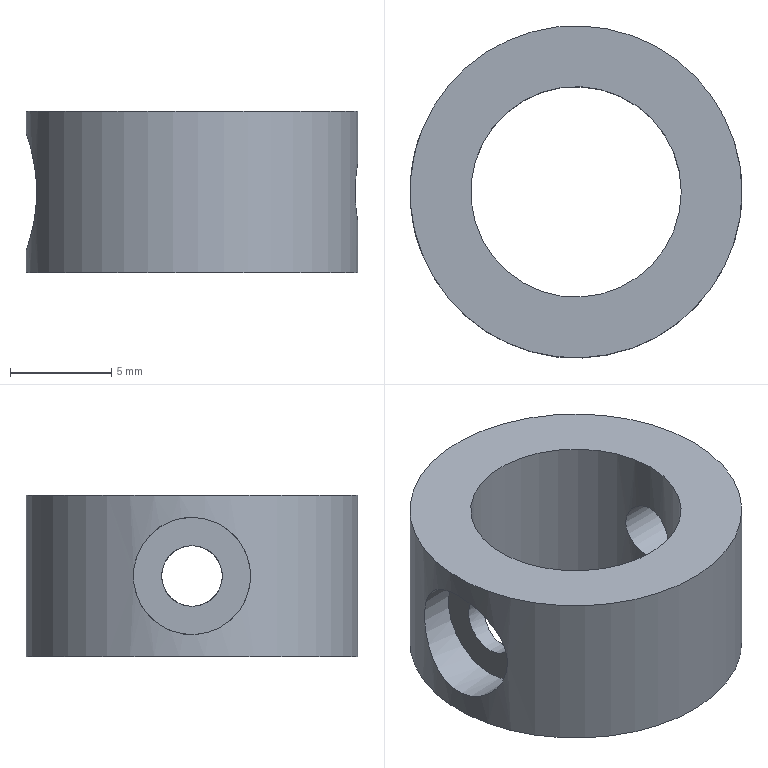Part | NX | features BREP 1, DATUM_CSYS 1 | 1 solid | 8 faces | box 16.4 x 16.4 x 8 mm | volume 928.38 mm3 | cylinder 5 | plane 3 | commonest cylinder face diameters 3 x2 5.8 x1 10.4 x1 16.4 x1
STEP:
#1=CARTESIAN_POINT('',(-6.,0.00000167,23.5));
#2=VERTEX_POINT('',#1);
#3=CARTESIAN_POINT('',(-6.,0.00000167,25.));
#4=DIRECTION('',(1.,0.,0.));
#5=DIRECTION('',(0.,0.,-1.));
#6=AXIS2_PLACEMENT_3D('',#3,#4,#5);
#7=CIRCLE('',#6,1.5);
#8=EDGE_CURVE('',#2,#2,#7,.T.);
#9=ORIENTED_EDGE('',*,*,#8,.F.);
#10=EDGE_LOOP('',(#9));
#11=FACE_BOUND('',#10,.T.);
#12=CARTESIAN_POINT('',(-5.2,-0.00002035,26.5));
#13=VERTEX_POINT('',#12);
#14=CARTESIAN_POINT('',(-5.092,-1.176,26.175));
#15=CARTESIAN_POINT('',(-5.254,0.0001171,26.663));
#16=CARTESIAN_POINT('',(-5.092,1.176,26.175));
#17=CARTESIAN_POINT('',(-4.922,1.662,25.002));
#18=CARTESIAN_POINT('',(-5.092,1.175,23.824));
#19=CARTESIAN_POINT('',(-5.254,0.0008864,23.338));
#20=CARTESIAN_POINT('',(-5.092,-1.175,23.824));
#21=CARTESIAN_POINT('',(-4.922,-1.662,25.));
#22=CARTESIAN_POINT('',(-5.092,-1.176,26.175));
#23=CARTESIAN_POINT('',(-5.254,0.0001171,26.663));
#24=CARTESIAN_POINT('',(-5.092,1.176,26.175));
#25=B_SPLINE_CURVE_WITH_KNOTS('',3,(#14,#15,#16,#17,#18,#19,#20,#21,#22,#23,#24),.UNSPECIFIED.,.T.,.F.,(1,1,1,1,1,1,1,1,1,1,1,1,1,1,1),(-0.003536,-0.002357,-0.001179,0.,0.001179,0.002357,0.003536,0.004714,0.005893,0.007071,0.00825,0.009428,0.01061,0.01179,0.01296),.UNSPECIFIED.);
#26=EDGE_CURVE('',#13,#13,#25,.T.);
#27=ORIENTED_EDGE('',*,*,#26,.F.);
#28=EDGE_LOOP('',(#27));
#29=FACE_BOUND('',#28,.T.);
#30=CARTESIAN_POINT('',(29.,0.00000167,25.));
#31=DIRECTION('',(-1.,0.,0.));
#32=DIRECTION('',(0.,0.,-1.));
#33=AXIS2_PLACEMENT_3D('',#30,#31,#32);
#34=CYLINDRICAL_SURFACE('',#33,1.5);
#35=ADVANCED_FACE('',(#11,#29),#34,.F.);
#36=CARTESIAN_POINT('',(5.2,0.00000167,26.5));
#37=VERTEX_POINT('',#36);
#38=CARTESIAN_POINT('',(5.092,1.176,26.175));
#39=CARTESIAN_POINT('',(5.254,-0.0001379,26.663));
#40=CARTESIAN_POINT('',(5.092,-1.176,26.174));
#41=CARTESIAN_POINT('',(4.923,-1.662,25.002));
#42=CARTESIAN_POINT('',(5.092,-1.175,23.824));
#43=CARTESIAN_POINT('',(5.254,-0.0008552,23.338));
#44=CARTESIAN_POINT('',(5.092,1.175,23.824));
#45=CARTESIAN_POINT('',(4.923,1.662,25.));
#46=CARTESIAN_POINT('',(5.092,1.176,26.175));
#47=CARTESIAN_POINT('',(5.254,-0.0001379,26.663));
#48=CARTESIAN_POINT('',(5.092,-1.176,26.174));
#49=B_SPLINE_CURVE_WITH_KNOTS('',3,(#38,#39,#40,#41,#42,#43,#44,#45,#46,#47,#48),.UNSPECIFIED.,.T.,.F.,(1,1,1,1,1,1,1,1,1,1,1,1,1,1,1),(-0.003536,-0.002357,-0.001179,0.,0.001179,0.002357,0.003536,0.004714,0.005893,0.007071,0.00825,0.009428,0.01061,0.01179,0.01296),.UNSPECIFIED.);
#50=EDGE_CURVE('',#37,#37,#49,.T.);
#51=ORIENTED_EDGE('',*,*,#50,.T.);
#52=EDGE_LOOP('',(#51));
#53=FACE_BOUND('',#52,.T.);
#54=CARTESIAN_POINT('',(5.2,-0.00002035,29.));
#55=VERTEX_POINT('',#54);
#56=CARTESIAN_POINT('',(0.0001029,-0.00002035,29.));
#57=DIRECTION('',(0.,0.,1.));
#58=DIRECTION('',(1.,0.,0.));
#59=AXIS2_PLACEMENT_3D('',#56,#57,#58);
#60=CIRCLE('',#59,5.2);
#61=EDGE_CURVE('',#55,#55,#60,.T.);
#62=ORIENTED_EDGE('',*,*,#61,.T.);
#63=EDGE_LOOP('',(#62));
#64=FACE_BOUND('',#63,.T.);
#65=CARTESIAN_POINT('',(5.2,-0.00002035,21.));
#66=VERTEX_POINT('',#65);
#67=CARTESIAN_POINT('',(0.0001029,-0.00002035,21.));
#68=DIRECTION('',(0.,0.,1.));
#69=DIRECTION('',(1.,0.,0.));
#70=AXIS2_PLACEMENT_3D('',#67,#68,#69);
#71=CIRCLE('',#70,5.2);
#72=EDGE_CURVE('',#66,#66,#71,.T.);
#73=ORIENTED_EDGE('',*,*,#72,.F.);
#74=EDGE_LOOP('',(#73));
#75=FACE_BOUND('',#74,.T.);
#76=ORIENTED_EDGE('',*,*,#26,.T.);
#77=EDGE_LOOP('',(#76));
#78=FACE_BOUND('',#77,.T.);
#79=CARTESIAN_POINT('',(0.0001029,-0.00002035,29.));
#80=DIRECTION('',(0.,0.,-1.));
#81=DIRECTION('',(1.,0.,0.));
#82=AXIS2_PLACEMENT_3D('',#79,#80,#81);
#83=CYLINDRICAL_SURFACE('',#82,5.2);
#84=ADVANCED_FACE('',(#53,#64,#75,#78),#83,.F.);
#85=CARTESIAN_POINT('',(-8.2,-0.00002035,27.9));
#86=VERTEX_POINT('',#85);
#87=CARTESIAN_POINT('',(-7.944,2.273,27.272));
#88=CARTESIAN_POINT('',(-8.328,0.0002532,28.215));
#89=CARTESIAN_POINT('',(-7.943,-2.274,27.27));
#90=CARTESIAN_POINT('',(-7.533,-3.214,25.004));
#91=CARTESIAN_POINT('',(-7.944,-2.272,22.726));
#92=CARTESIAN_POINT('',(-8.328,-0.002018,21.787));
#93=CARTESIAN_POINT('',(-7.944,2.274,22.728));
#94=CARTESIAN_POINT('',(-7.533,3.213,25.001));
#95=CARTESIAN_POINT('',(-7.944,2.273,27.272));
#96=CARTESIAN_POINT('',(-8.328,0.0002532,28.215));
#97=CARTESIAN_POINT('',(-7.943,-2.274,27.27));
#98=B_SPLINE_CURVE_WITH_KNOTS('',3,(#87,#88,#89,#90,#91,#92,#93,#94,#95,#96,#97),.UNSPECIFIED.,.T.,.F.,(1,1,1,1,1,1,1,1,1,1,1,1,1,1,1),(-0.006855,-0.00457,-0.002285,0.,0.002285,0.00457,0.006855,0.00914,0.01143,0.01371,0.016,0.01828,0.02057,0.02285,0.02514),.UNSPECIFIED.);
#99=EDGE_CURVE('',#86,#86,#98,.T.);
#100=ORIENTED_EDGE('',*,*,#99,.T.);
#101=EDGE_LOOP('',(#100));
#102=FACE_BOUND('',#101,.T.);
#103=CARTESIAN_POINT('',(8.2,-0.00002035,29.));
#104=VERTEX_POINT('',#103);
#105=CARTESIAN_POINT('',(0.0001029,-0.00002035,29.));
#106=DIRECTION('',(0.,0.,1.));
#107=DIRECTION('',(1.,0.,0.));
#108=AXIS2_PLACEMENT_3D('',#105,#106,#107);
#109=CIRCLE('',#108,8.2);
#110=EDGE_CURVE('',#104,#104,#109,.T.);
#111=ORIENTED_EDGE('',*,*,#110,.F.);
#112=EDGE_LOOP('',(#111));
#113=FACE_BOUND('',#112,.T.);
#114=CARTESIAN_POINT('',(8.2,-0.00002035,21.));
#115=VERTEX_POINT('',#114);
#116=CARTESIAN_POINT('',(0.0001029,-0.00002035,21.));
#117=DIRECTION('',(0.,0.,1.));
#118=DIRECTION('',(1.,0.,0.));
#119=AXIS2_PLACEMENT_3D('',#116,#117,#118);
#120=CIRCLE('',#119,8.2);
#121=EDGE_CURVE('',#115,#115,#120,.T.);
#122=ORIENTED_EDGE('',*,*,#121,.T.);
#123=EDGE_LOOP('',(#122));
#124=FACE_BOUND('',#123,.T.);
#125=CARTESIAN_POINT('',(8.2,0.00000167,26.5));
#126=VERTEX_POINT('',#125);
#127=CARTESIAN_POINT('',(8.131,1.177,26.174));
#128=CARTESIAN_POINT('',(8.234,-0.00027,26.663));
#129=CARTESIAN_POINT('',(8.131,-1.176,26.175));
#130=CARTESIAN_POINT('',(8.027,-1.662,25.002));
#131=CARTESIAN_POINT('',(8.131,-1.176,23.825));
#132=CARTESIAN_POINT('',(8.234,-0.0004839,23.338));
#133=CARTESIAN_POINT('',(8.132,1.174,23.823));
#134=CARTESIAN_POINT('',(8.027,1.662,24.999));
#135=CARTESIAN_POINT('',(8.131,1.177,26.174));
#136=CARTESIAN_POINT('',(8.234,-0.00027,26.663));
#137=CARTESIAN_POINT('',(8.131,-1.176,26.175));
#138=B_SPLINE_CURVE_WITH_KNOTS('',3,(#127,#128,#129,#130,#131,#132,#133,#134,#135,#136,#137),.UNSPECIFIED.,.T.,.F.,(1,1,1,1,1,1,1,1,1,1,1,1,1,1,1),(-0.003524,-0.002349,-0.001175,0.,0.001175,0.002349,0.003524,0.004699,0.005874,0.007048,0.008223,0.009398,0.01057,0.01175,0.01292),.UNSPECIFIED.);
#139=EDGE_CURVE('',#126,#126,#138,.T.);
#140=ORIENTED_EDGE('',*,*,#139,.F.);
#141=EDGE_LOOP('',(#140));
#142=FACE_BOUND('',#141,.T.);
#143=CARTESIAN_POINT('',(0.0001029,-0.00002035,29.));
#144=DIRECTION('',(0.,0.,-1.));
#145=DIRECTION('',(1.,0.,0.));
#146=AXIS2_PLACEMENT_3D('',#143,#144,#145);
#147=CYLINDRICAL_SURFACE('',#146,8.2);
#148=ADVANCED_FACE('',(#102,#113,#124,#142),#147,.T.);
#149=ORIENTED_EDGE('',*,*,#72,.T.);
#150=EDGE_LOOP('',(#149));
#151=FACE_BOUND('',#150,.T.);
#152=ORIENTED_EDGE('',*,*,#121,.F.);
#153=EDGE_LOOP('',(#152));
#154=FACE_BOUND('',#153,.T.);
#155=CARTESIAN_POINT('',(0.,0.,21.));
#156=DIRECTION('',(0.,0.,1.));
#157=DIRECTION('',(-1.,0.,0.));
#158=AXIS2_PLACEMENT_3D('',#155,#156,#157);
#159=PLANE('',#158);
#160=ADVANCED_FACE('',(#151,#154),#159,.F.);
#161=ORIENTED_EDGE('',*,*,#50,.F.);
#162=EDGE_LOOP('',(#161));
#163=FACE_BOUND('',#162,.T.);
#164=ORIENTED_EDGE('',*,*,#139,.T.);
#165=EDGE_LOOP('',(#164));
#166=FACE_BOUND('',#165,.T.);
#167=CARTESIAN_POINT('',(29.,0.00000167,25.));
#168=DIRECTION('',(-1.,0.,0.));
#169=DIRECTION('',(0.,0.,-1.));
#170=AXIS2_PLACEMENT_3D('',#167,#168,#169);
#171=CYLINDRICAL_SURFACE('',#170,1.5);
#172=ADVANCED_FACE('',(#163,#166),#171,.F.);
#173=ORIENTED_EDGE('',*,*,#61,.F.);
#174=EDGE_LOOP('',(#173));
#175=FACE_BOUND('',#174,.T.);
#176=ORIENTED_EDGE('',*,*,#110,.T.);
#177=EDGE_LOOP('',(#176));
#178=FACE_BOUND('',#177,.T.);
#179=CARTESIAN_POINT('',(0.,0.,29.));
#180=DIRECTION('',(0.,0.,1.));
#181=DIRECTION('',(-1.,0.,0.));
#182=AXIS2_PLACEMENT_3D('',#179,#180,#181);
#183=PLANE('',#182);
#184=ADVANCED_FACE('',(#175,#178),#183,.T.);
#185=ORIENTED_EDGE('',*,*,#8,.T.);
#186=EDGE_LOOP('',(#185));
#187=FACE_BOUND('',#186,.T.);
#188=CARTESIAN_POINT('',(-6.,0.00001842,22.1));
#189=VERTEX_POINT('',#188);
#190=CARTESIAN_POINT('',(-6.,0.00001842,25.));
#191=DIRECTION('',(1.,0.,0.));
#192=DIRECTION('',(0.,0.,-1.));
#193=AXIS2_PLACEMENT_3D('',#190,#191,#192);
#194=CIRCLE('',#193,2.9);
#195=EDGE_CURVE('',#189,#189,#194,.T.);
#196=ORIENTED_EDGE('',*,*,#195,.F.);
#197=EDGE_LOOP('',(#196));
#198=FACE_BOUND('',#197,.T.);
#199=CARTESIAN_POINT('',(-6.,0.,0.));
#200=DIRECTION('',(1.,0.,0.));
#201=DIRECTION('',(0.,0.,1.));
#202=AXIS2_PLACEMENT_3D('',#199,#200,#201);
#203=PLANE('',#202);
#204=ADVANCED_FACE('',(#187,#198),#203,.F.);
#205=ORIENTED_EDGE('',*,*,#195,.T.);
#206=EDGE_LOOP('',(#205));
#207=FACE_BOUND('',#206,.T.);
#208=ORIENTED_EDGE('',*,*,#99,.F.);
#209=EDGE_LOOP('',(#208));
#210=FACE_BOUND('',#209,.T.);
#211=CARTESIAN_POINT('',(-14.2,0.00001842,25.));
#212=DIRECTION('',(1.,0.,0.));
#213=DIRECTION('',(0.,0.,1.));
#214=AXIS2_PLACEMENT_3D('',#211,#212,#213);
#215=CYLINDRICAL_SURFACE('',#214,2.9);
#216=ADVANCED_FACE('',(#207,#210),#215,.F.);
#217=CLOSED_SHELL('',(#35,#84,#148,#160,#172,#184,#204,#216));
#218=MANIFOLD_SOLID_BREP('',#217);
#219=(LENGTH_UNIT()NAMED_UNIT(*)SI_UNIT(.MILLI.,.METRE.));
#220=UNCERTAINTY_MEASURE_WITH_UNIT(LENGTH_MEASURE(0.0508),#219,'','');
#221=(NAMED_UNIT(*)PLANE_ANGLE_UNIT()SI_UNIT($,.RADIAN.));
#222=(NAMED_UNIT(*)SI_UNIT($,.STERADIAN.)SOLID_ANGLE_UNIT());
#223=(GEOMETRIC_REPRESENTATION_CONTEXT(3)GLOBAL_UNCERTAINTY_ASSIGNED_CONTEXT((#220))GLOBAL_UNIT_ASSIGNED_CONTEXT((#219,#221,#222))REPRESENTATION_CONTEXT('',''));
#224=ADVANCED_BREP_SHAPE_REPRESENTATION('',(#218),#223);